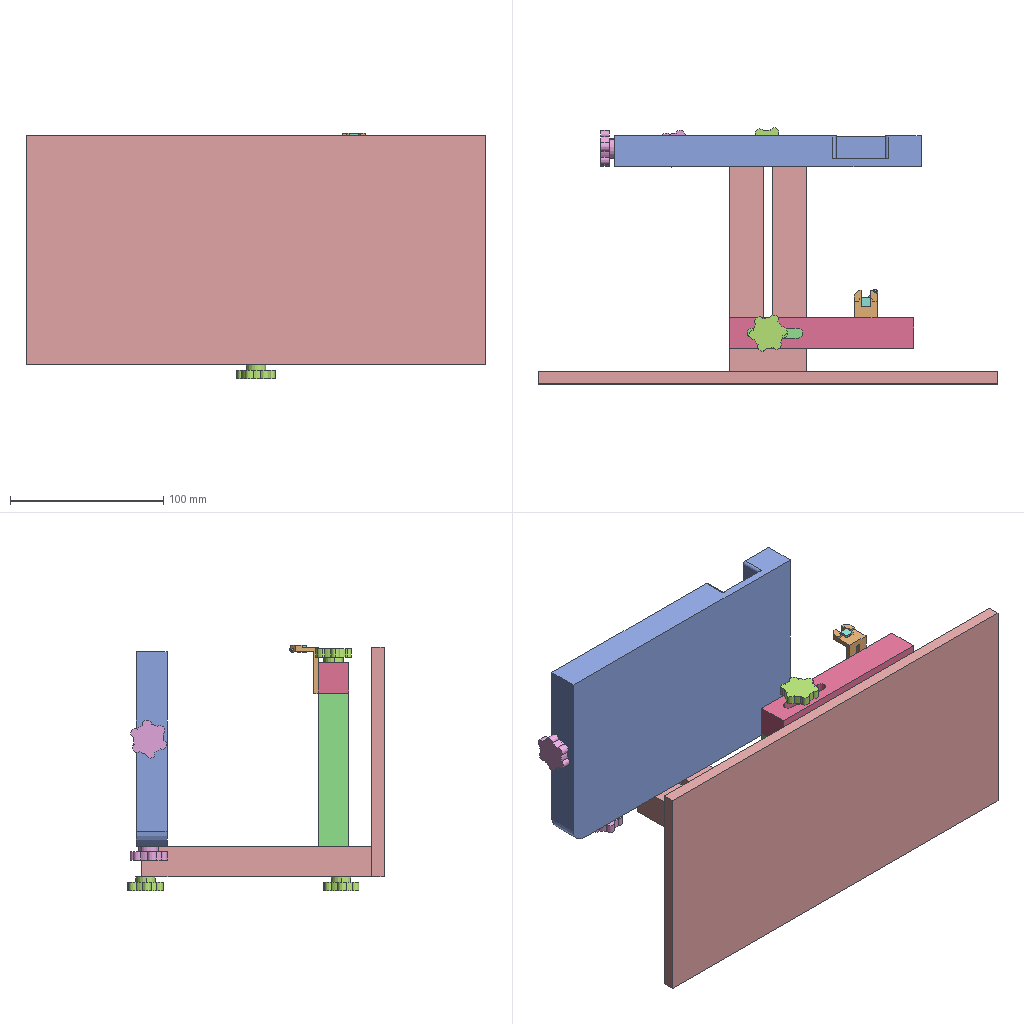Assembly | SolidWorks | 10 different items | 13 placed | box 300 x 167 x 160 mm
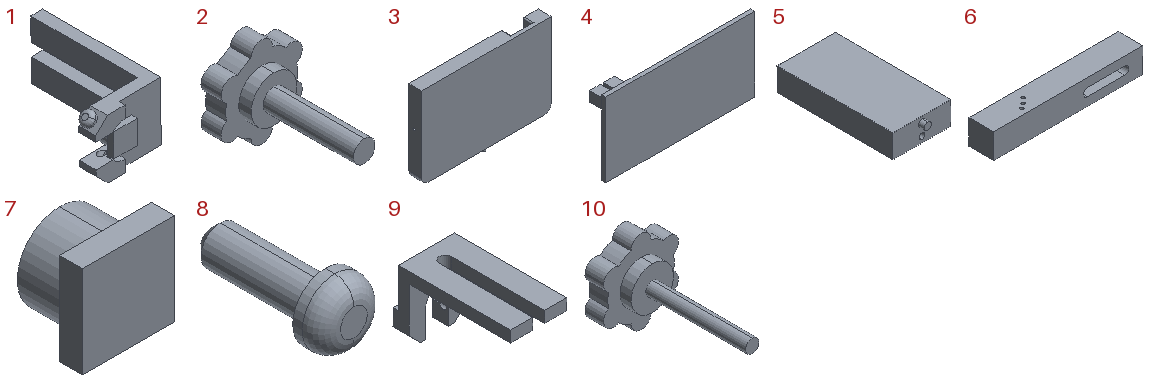Parts list (item | name | quantity | parent item | size | volume | features):
1 | (subassembly) | x1 | - | 18.773 x 31.5 x 15.421 mm | 1749 mm3 | -
2 | - | x3 | - | 22.455 x 34 x 25 mm | 3296 mm3 | features ICE 2, Extrusion 1
3 | - | x1 | - | 200 x 20 x 131.788 mm | 297123 mm3 | features ICE 4, Fillet 3, HoleWzd 3, Extrusion 1
4 | - | x1 | - | 300 x 158 x 150 mm | 493578 mm3 | features ICE 2, Extrusion 1
5 | - | x1 | - | 50 x 110 x 20 mm | 99674 mm3 | features ICE 4, HoleWzd 3, Extrusion 1
6 | - | x1 | - | 120 x 20 x 20 mm | 43402 mm3 | features ICE 5, HoleWzd 2, Extrusion 1
7 | - | x1 | in 1 | 6 x 4.5 x 6 mm | 125.275 mm3 | features Extrusion 1, ICE 1
8 | - | x1 | in 1 | 3.4 x 7.5 x 3.4 mm | 29.823 mm3 | features Chamfer 1, Extrusion 1, Fillet 1, ICE 1
9 | - | x1 | in 1 | 15 x 31.5 x 18 mm | 1594 mm3 | features ICE 6, Extrusion 1, HoleWzd 1, MirrorPattern 1
10 | - | x2 | - | 22.455 x 39 x 25 mm | 2966 mm3 | features ICE 2, Extrusion 1
Mates (type | each side: item.copy, entity, surface, feature):
In the top assembly
Coincident | 4.1 face plane Boss-Extrude2 | 3.1 face plane Boss-Extrude1
Tangent | 4.1 face plane Cut-Extrude1 | 3.1 face cylinder Boss-Extrude2
Parallel | 4.1 face plane Boss-Extrude1 | 3.1 face plane Boss-Extrude1
Concentric | 3.1 face cylinder M6 Tapped Hole1 | 2.1 face cylinder Boss-Extrude2
Coincident | 4.1 face plane Boss-Extrude1 | 2.1 face plane Boss-Extrude2
Concentric | 3.1 face cylinder M4 Tapped Hole1 | 10.1 face cylinder Boss-Extrude3
Coincident | 3.1 face plane Boss-Extrude1 | 10.1 face plane Boss-Extrude2
Concentric | 3.1 face cylinder M4 Tapped Hole2 | 10.2 face cylinder Boss-Extrude3
Coincident | 3.1 face plane Boss-Extrude1 | 10.2 face plane Boss-Extrude2
Concentric | 4.1 face cylinder Cut-Extrude1 | 5.1 face cylinder M6 Tapped Hole1
Coincident | 4.1 face plane Boss-Extrude2 | 5.1 face plane Boss-Extrude1
Parallel | 4.1 face plane Boss-Extrude1 | 5.1 face plane Boss-Extrude1
Concentric | 5.1 face cylinder M6 Tapped Hole1 | 2.2 face cylinder Boss-Extrude3
Coincident | 4.1 face plane Boss-Extrude1 | 2.2 face plane Boss-Extrude2
Coincident | 9.1 face plane Boss-Extrude4 | 5.1 face plane Boss-Extrude1
Coincident | 5.1 face plane Cut-Extrude1 | 6.1 face plane Boss-Extrude3
Coincident | 5.1 face plane Boss-Extrude1 | 6.1 face plane Boss-Extrude1 | 2 times
Concentric | 5.1 face cylinder M6 Tapped Hole2 | 2.3 face cylinder Boss-Extrude3
Coincident | 6.1 face plane Cut-Extrude3 | 2.3 face plane Boss-Extrude2
In subassembly 1
Concentric | 7.1 face cylinder Boss-Extrude1 | 9.2 face cylinder Boss-Extrude1
Coincident | 7.1 face plane Boss-Extrude2 | 9.2 face plane Boss-Extrude1
Concentric | 9.2 face cylinder M2 Tapped Hole1 | 8.1 face cylinder Boss-Extrude1